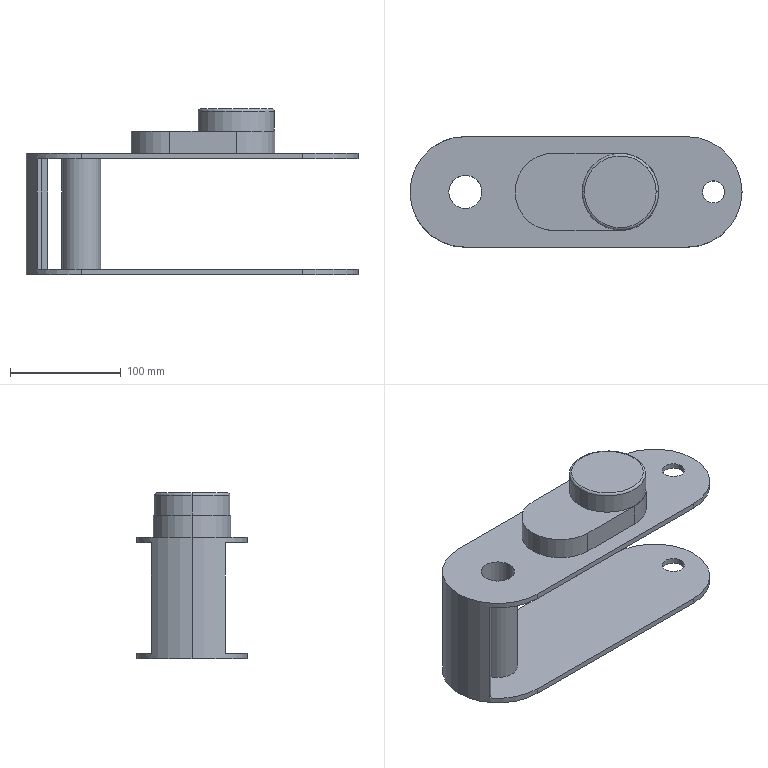Part | SolidWorks | features ICE 7, Extrusion 1, Fillet 1 | 1 solid | 41 faces | box 300 x 100 x 150 mm | volume 561268 mm3 | cylinder 23 | plane 16 | torus 2 | commonest cylinder face diameters 20 x8 100 x4 70 x3 30 x2 35 x2 69 x2
STEP:
#1=CARTESIAN_POINT('',(105.5,0.,148.));
#2=VERTEX_POINT('',#1);
#3=CARTESIAN_POINT('',(174.5,0.,148.));
#4=VERTEX_POINT('',#3);
#5=CARTESIAN_POINT('',(140.,0.,148.));
#6=DIRECTION('',(0.,0.,-1.));
#7=DIRECTION('',(1.,0.,0.));
#8=AXIS2_PLACEMENT_3D('',#5,#6,#7);
#9=CIRCLE('',#8,34.5);
#10=EDGE_CURVE('',#2,#4,#9,.T.);
#11=ORIENTED_EDGE('',*,*,#10,.F.);
#12=CARTESIAN_POINT('',(107.5,0.,150.));
#13=VERTEX_POINT('',#12);
#14=CARTESIAN_POINT('',(107.5,0.,148.));
#15=DIRECTION('',(0.,1.,0.));
#16=DIRECTION('',(-1.,0.,0.));
#17=AXIS2_PLACEMENT_3D('',#14,#15,#16);
#18=CIRCLE('',#17,2.);
#19=EDGE_CURVE('',#2,#13,#18,.T.);
#20=ORIENTED_EDGE('',*,*,#19,.T.);
#21=CARTESIAN_POINT('',(172.5,0.,150.));
#22=VERTEX_POINT('',#21);
#23=CARTESIAN_POINT('',(140.,0.,150.));
#24=DIRECTION('',(0.,0.,1.));
#25=DIRECTION('',(1.,0.,0.));
#26=AXIS2_PLACEMENT_3D('',#23,#24,#25);
#27=CIRCLE('',#26,32.5);
#28=EDGE_CURVE('',#22,#13,#27,.T.);
#29=ORIENTED_EDGE('',*,*,#28,.F.);
#30=CARTESIAN_POINT('',(172.5,0.,148.));
#31=DIRECTION('',(0.,-1.,0.));
#32=DIRECTION('',(0.,0.,-1.));
#33=AXIS2_PLACEMENT_3D('',#30,#31,#32);
#34=CIRCLE('',#33,2.);
#35=EDGE_CURVE('',#4,#22,#34,.T.);
#36=ORIENTED_EDGE('',*,*,#35,.F.);
#37=EDGE_LOOP('',(#11,#20,#29,#36));
#38=FACE_OUTER_BOUND('',#37,.T.);
#39=CARTESIAN_POINT('',(140.,0.,148.));
#40=DIRECTION('',(0.,0.,1.));
#41=DIRECTION('',(1.,0.,0.));
#42=AXIS2_PLACEMENT_3D('',#39,#40,#41);
#43=TOROIDAL_SURFACE('',#42,32.5,2.);
#44=ADVANCED_FACE('',(#38),#43,.T.);
#45=CARTESIAN_POINT('',(-45.,0.,105.));
#46=VERTEX_POINT('',#45);
#47=CARTESIAN_POINT('',(-30.342,33.232,105.));
#48=VERTEX_POINT('',#47);
#49=CARTESIAN_POINT('',(0.,0.,105.));
#50=DIRECTION('',(0.,0.,-1.));
#51=DIRECTION('',(1.,0.,0.));
#52=AXIS2_PLACEMENT_3D('',#49,#50,#51);
#53=CIRCLE('',#52,45.);
#54=EDGE_CURVE('',#46,#48,#53,.T.);
#55=ORIENTED_EDGE('',*,*,#54,.F.);
#56=CARTESIAN_POINT('',(-45.,0.,5.));
#57=VERTEX_POINT('',#56);
#58=CARTESIAN_POINT('',(-45.,0.,150.002));
#59=DIRECTION('',(0.,0.,-1.));
#60=VECTOR('',#59,1000.);
#61=LINE('',#58,#60);
#62=EDGE_CURVE('',#46,#57,#61,.T.);
#63=ORIENTED_EDGE('',*,*,#62,.T.);
#64=CARTESIAN_POINT('',(-30.342,33.232,5.));
#65=VERTEX_POINT('',#64);
#66=CARTESIAN_POINT('',(0.,0.,5.));
#67=DIRECTION('',(0.,0.,-1.));
#68=DIRECTION('',(1.,0.,0.));
#69=AXIS2_PLACEMENT_3D('',#66,#67,#68);
#70=CIRCLE('',#69,45.);
#71=EDGE_CURVE('',#57,#65,#70,.T.);
#72=ORIENTED_EDGE('',*,*,#71,.T.);
#73=CARTESIAN_POINT('',(-30.342,33.232,150.002));
#74=DIRECTION('',(0.,0.,-1.));
#75=VECTOR('',#74,1000.);
#76=LINE('',#73,#75);
#77=EDGE_CURVE('',#48,#65,#76,.T.);
#78=ORIENTED_EDGE('',*,*,#77,.F.);
#79=EDGE_LOOP('',(#55,#63,#72,#78));
#80=FACE_OUTER_BOUND('',#79,.T.);
#81=CARTESIAN_POINT('',(0.,0.,150.002));
#82=DIRECTION('',(0.,0.,-1.));
#83=DIRECTION('',(-1.,0.,0.));
#84=AXIS2_PLACEMENT_3D('',#81,#82,#83);
#85=CYLINDRICAL_SURFACE('',#84,45.);
#86=ADVANCED_FACE('',(#80),#85,.F.);
#87=CARTESIAN_POINT('',(214.307,0.,5.));
#88=VERTEX_POINT('',#87);
#89=CARTESIAN_POINT('',(234.307,0.,5.));
#90=VERTEX_POINT('',#89);
#91=CARTESIAN_POINT('',(224.307,0.,5.));
#92=DIRECTION('',(0.,0.,1.));
#93=DIRECTION('',(1.,0.,0.));
#94=AXIS2_PLACEMENT_3D('',#91,#92,#93);
#95=CIRCLE('',#94,10.);
#96=EDGE_CURVE('',#88,#90,#95,.T.);
#97=ORIENTED_EDGE('',*,*,#96,.T.);
#98=CARTESIAN_POINT('',(234.307,0.,0.));
#99=VERTEX_POINT('',#98);
#100=CARTESIAN_POINT('',(234.307,0.,127.));
#101=DIRECTION('',(0.,0.,-1.));
#102=VECTOR('',#101,1000.);
#103=LINE('',#100,#102);
#104=EDGE_CURVE('',#90,#99,#103,.T.);
#105=ORIENTED_EDGE('',*,*,#104,.T.);
#106=CARTESIAN_POINT('',(214.307,0.,0.));
#107=VERTEX_POINT('',#106);
#108=CARTESIAN_POINT('',(224.307,0.,0.));
#109=DIRECTION('',(0.,0.,-1.));
#110=DIRECTION('',(-1.,0.,0.));
#111=AXIS2_PLACEMENT_3D('',#108,#109,#110);
#112=CIRCLE('',#111,10.);
#113=EDGE_CURVE('',#99,#107,#112,.T.);
#114=ORIENTED_EDGE('',*,*,#113,.T.);
#115=CARTESIAN_POINT('',(214.307,0.,127.));
#116=DIRECTION('',(0.,0.,-1.));
#117=VECTOR('',#116,1000.);
#118=LINE('',#115,#117);
#119=EDGE_CURVE('',#88,#107,#118,.T.);
#120=ORIENTED_EDGE('',*,*,#119,.F.);
#121=EDGE_LOOP('',(#97,#105,#114,#120));
#122=FACE_OUTER_BOUND('',#121,.T.);
#123=CARTESIAN_POINT('',(224.307,0.,127.));
#124=DIRECTION('',(0.,0.,-1.));
#125=DIRECTION('',(-1.,0.,0.));
#126=AXIS2_PLACEMENT_3D('',#123,#124,#125);
#127=CYLINDRICAL_SURFACE('',#126,10.);
#128=ADVANCED_FACE('',(#122),#127,.F.);
#129=CARTESIAN_POINT('',(214.307,0.,110.));
#130=VERTEX_POINT('',#129);
#131=CARTESIAN_POINT('',(234.307,0.,110.));
#132=VERTEX_POINT('',#131);
#133=CARTESIAN_POINT('',(224.307,0.,110.));
#134=DIRECTION('',(0.,0.,1.));
#135=DIRECTION('',(1.,0.,0.));
#136=AXIS2_PLACEMENT_3D('',#133,#134,#135);
#137=CIRCLE('',#136,10.);
#138=EDGE_CURVE('',#130,#132,#137,.T.);
#139=ORIENTED_EDGE('',*,*,#138,.T.);
#140=CARTESIAN_POINT('',(234.307,0.,105.));
#141=VERTEX_POINT('',#140);
#142=CARTESIAN_POINT('',(234.307,0.,127.));
#143=DIRECTION('',(0.,0.,-1.));
#144=VECTOR('',#143,1000.);
#145=LINE('',#142,#144);
#146=EDGE_CURVE('',#132,#141,#145,.T.);
#147=ORIENTED_EDGE('',*,*,#146,.T.);
#148=CARTESIAN_POINT('',(214.307,0.,105.));
#149=VERTEX_POINT('',#148);
#150=CARTESIAN_POINT('',(224.307,0.,105.));
#151=DIRECTION('',(0.,0.,1.));
#152=DIRECTION('',(1.,0.,0.));
#153=AXIS2_PLACEMENT_3D('',#150,#151,#152);
#154=CIRCLE('',#153,10.);
#155=EDGE_CURVE('',#149,#141,#154,.T.);
#156=ORIENTED_EDGE('',*,*,#155,.F.);
#157=CARTESIAN_POINT('',(214.307,0.,127.));
#158=DIRECTION('',(0.,0.,-1.));
#159=VECTOR('',#158,1000.);
#160=LINE('',#157,#159);
#161=EDGE_CURVE('',#130,#149,#160,.T.);
#162=ORIENTED_EDGE('',*,*,#161,.F.);
#163=EDGE_LOOP('',(#139,#147,#156,#162));
#164=FACE_OUTER_BOUND('',#163,.T.);
#165=CARTESIAN_POINT('',(224.307,0.,127.));
#166=DIRECTION('',(0.,0.,-1.));
#167=DIRECTION('',(-1.,0.,0.));
#168=AXIS2_PLACEMENT_3D('',#165,#166,#167);
#169=CYLINDRICAL_SURFACE('',#168,10.);
#170=ADVANCED_FACE('',(#164),#169,.F.);
#171=ORIENTED_EDGE('',*,*,#10,.T.);
#172=CARTESIAN_POINT('',(174.5,0.,130.));
#173=VERTEX_POINT('',#172);
#174=CARTESIAN_POINT('',(174.5,0.,150.));
#175=DIRECTION('',(0.,0.,-1.));
#176=VECTOR('',#175,1000.);
#177=LINE('',#174,#176);
#178=EDGE_CURVE('',#4,#173,#177,.T.);
#179=ORIENTED_EDGE('',*,*,#178,.T.);
#180=CARTESIAN_POINT('',(105.5,0.,130.));
#181=VERTEX_POINT('',#180);
#182=CARTESIAN_POINT('',(140.,0.,130.));
#183=DIRECTION('',(0.,0.,1.));
#184=DIRECTION('',(1.,0.,0.));
#185=AXIS2_PLACEMENT_3D('',#182,#183,#184);
#186=CIRCLE('',#185,34.5);
#187=EDGE_CURVE('',#173,#181,#186,.T.);
#188=ORIENTED_EDGE('',*,*,#187,.T.);
#189=CARTESIAN_POINT('',(105.5,0.,150.));
#190=DIRECTION('',(0.,0.,-1.));
#191=VECTOR('',#190,1000.);
#192=LINE('',#189,#191);
#193=EDGE_CURVE('',#2,#181,#192,.T.);
#194=ORIENTED_EDGE('',*,*,#193,.F.);
#195=EDGE_LOOP('',(#171,#179,#188,#194));
#196=FACE_OUTER_BOUND('',#195,.T.);
#197=CARTESIAN_POINT('',(140.,0.,150.));
#198=DIRECTION('',(0.,0.,-1.));
#199=DIRECTION('',(-1.,0.,0.));
#200=AXIS2_PLACEMENT_3D('',#197,#198,#199);
#201=CYLINDRICAL_SURFACE('',#200,34.5);
#202=ADVANCED_FACE('',(#196),#201,.T.);
#203=CARTESIAN_POINT('',(45.,0.,130.));
#204=VERTEX_POINT('',#203);
#205=CARTESIAN_POINT('',(80.,-35.,130.));
#206=VERTEX_POINT('',#205);
#207=CARTESIAN_POINT('',(80.,0.,130.));
#208=DIRECTION('',(0.,0.,1.));
#209=DIRECTION('',(1.,0.,0.));
#210=AXIS2_PLACEMENT_3D('',#207,#208,#209);
#211=CIRCLE('',#210,35.);
#212=EDGE_CURVE('',#204,#206,#211,.T.);
#213=ORIENTED_EDGE('',*,*,#212,.F.);
#214=CARTESIAN_POINT('',(45.,0.,110.));
#215=VERTEX_POINT('',#214);
#216=CARTESIAN_POINT('',(45.,0.,130.));
#217=DIRECTION('',(0.,0.,-1.));
#218=VECTOR('',#217,1000.);
#219=LINE('',#216,#218);
#220=EDGE_CURVE('',#204,#215,#219,.T.);
#221=ORIENTED_EDGE('',*,*,#220,.T.);
#222=CARTESIAN_POINT('',(80.,-35.,110.));
#223=VERTEX_POINT('',#222);
#224=CARTESIAN_POINT('',(80.,0.,110.));
#225=DIRECTION('',(0.,0.,1.));
#226=DIRECTION('',(1.,0.,0.));
#227=AXIS2_PLACEMENT_3D('',#224,#225,#226);
#228=CIRCLE('',#227,35.);
#229=EDGE_CURVE('',#215,#223,#228,.T.);
#230=ORIENTED_EDGE('',*,*,#229,.T.);
#231=CARTESIAN_POINT('',(80.,-35.,130.));
#232=DIRECTION('',(0.,0.,-1.));
#233=VECTOR('',#232,1000.);
#234=LINE('',#231,#233);
#235=EDGE_CURVE('',#206,#223,#234,.T.);
#236=ORIENTED_EDGE('',*,*,#235,.F.);
#237=EDGE_LOOP('',(#213,#221,#230,#236));
#238=FACE_OUTER_BOUND('',#237,.T.);
#239=CARTESIAN_POINT('',(80.,0.,130.));
#240=DIRECTION('',(0.,0.,-1.));
#241=DIRECTION('',(-1.,0.,0.));
#242=AXIS2_PLACEMENT_3D('',#239,#240,#241);
#243=CYLINDRICAL_SURFACE('',#242,35.);
#244=ADVANCED_FACE('',(#238),#243,.T.);
#245=CARTESIAN_POINT('',(130.,0.,110.));
#246=VERTEX_POINT('',#245);
#247=CARTESIAN_POINT('',(150.,0.,110.));
#248=VERTEX_POINT('',#247);
#249=CARTESIAN_POINT('',(140.,0.,110.));
#250=DIRECTION('',(0.,0.,1.));
#251=DIRECTION('',(1.,0.,0.));
#252=AXIS2_PLACEMENT_3D('',#249,#250,#251);
#253=CIRCLE('',#252,10.);
#254=EDGE_CURVE('',#246,#248,#253,.T.);
#255=ORIENTED_EDGE('',*,*,#254,.T.);
#256=CARTESIAN_POINT('',(150.,0.,105.));
#257=VERTEX_POINT('',#256);
#258=CARTESIAN_POINT('',(150.,0.,151.));
#259=DIRECTION('',(0.,0.,-1.));
#260=VECTOR('',#259,1000.);
#261=LINE('',#258,#260);
#262=EDGE_CURVE('',#248,#257,#261,.T.);
#263=ORIENTED_EDGE('',*,*,#262,.T.);
#264=CARTESIAN_POINT('',(130.,0.,105.));
#265=VERTEX_POINT('',#264);
#266=CARTESIAN_POINT('',(140.,0.,105.));
#267=DIRECTION('',(0.,0.,-1.));
#268=DIRECTION('',(-1.,0.,0.));
#269=AXIS2_PLACEMENT_3D('',#266,#267,#268);
#270=CIRCLE('',#269,10.);
#271=EDGE_CURVE('',#257,#265,#270,.T.);
#272=ORIENTED_EDGE('',*,*,#271,.T.);
#273=CARTESIAN_POINT('',(130.,0.,151.));
#274=DIRECTION('',(0.,0.,-1.));
#275=VECTOR('',#274,1000.);
#276=LINE('',#273,#275);
#277=EDGE_CURVE('',#246,#265,#276,.T.);
#278=ORIENTED_EDGE('',*,*,#277,.F.);
#279=EDGE_LOOP('',(#255,#263,#272,#278));
#280=FACE_OUTER_BOUND('',#279,.T.);
#281=CARTESIAN_POINT('',(140.,0.,151.));
#282=DIRECTION('',(0.,0.,-1.));
#283=DIRECTION('',(-1.,0.,0.));
#284=AXIS2_PLACEMENT_3D('',#281,#282,#283);
#285=CYLINDRICAL_SURFACE('',#284,10.);
#286=ADVANCED_FACE('',(#280),#285,.F.);
#287=CARTESIAN_POINT('',(70.,0.,110.));
#288=VERTEX_POINT('',#287);
#289=CARTESIAN_POINT('',(90.,0.,110.));
#290=VERTEX_POINT('',#289);
#291=CARTESIAN_POINT('',(80.,0.,110.));
#292=DIRECTION('',(0.,0.,1.));
#293=DIRECTION('',(1.,0.,0.));
#294=AXIS2_PLACEMENT_3D('',#291,#292,#293);
#295=CIRCLE('',#294,10.);
#296=EDGE_CURVE('',#288,#290,#295,.T.);
#297=ORIENTED_EDGE('',*,*,#296,.T.);
#298=CARTESIAN_POINT('',(90.,0.,105.));
#299=VERTEX_POINT('',#298);
#300=CARTESIAN_POINT('',(90.,0.,151.));
#301=DIRECTION('',(0.,0.,-1.));
#302=VECTOR('',#301,1000.);
#303=LINE('',#300,#302);
#304=EDGE_CURVE('',#290,#299,#303,.T.);
#305=ORIENTED_EDGE('',*,*,#304,.T.);
#306=CARTESIAN_POINT('',(70.,0.,105.));
#307=VERTEX_POINT('',#306);
#308=CARTESIAN_POINT('',(80.,0.,105.));
#309=DIRECTION('',(0.,0.,-1.));
#310=DIRECTION('',(-1.,0.,0.));
#311=AXIS2_PLACEMENT_3D('',#308,#309,#310);
#312=CIRCLE('',#311,10.);
#313=EDGE_CURVE('',#299,#307,#312,.T.);
#314=ORIENTED_EDGE('',*,*,#313,.T.);
#315=CARTESIAN_POINT('',(70.,0.,151.));
#316=DIRECTION('',(0.,0.,-1.));
#317=VECTOR('',#316,1000.);
#318=LINE('',#315,#317);
#319=EDGE_CURVE('',#288,#307,#318,.T.);
#320=ORIENTED_EDGE('',*,*,#319,.F.);
#321=EDGE_LOOP('',(#297,#305,#314,#320));
#322=FACE_OUTER_BOUND('',#321,.T.);
#323=CARTESIAN_POINT('',(80.,0.,151.));
#324=DIRECTION('',(0.,0.,-1.));
#325=DIRECTION('',(-1.,0.,0.));
#326=AXIS2_PLACEMENT_3D('',#323,#324,#325);
#327=CYLINDRICAL_SURFACE('',#326,10.);
#328=ADVANCED_FACE('',(#322),#327,.F.);
#329=CARTESIAN_POINT('',(17.5,0.,105.));
#330=VERTEX_POINT('',#329);
#331=CARTESIAN_POINT('',(-17.5,0.,105.));
#332=VERTEX_POINT('',#331);
#333=CARTESIAN_POINT('',(0.,0.,105.));
#334=DIRECTION('',(0.,0.,1.));
#335=DIRECTION('',(1.,0.,0.));
#336=AXIS2_PLACEMENT_3D('',#333,#334,#335);
#337=CIRCLE('',#336,17.5);
#338=EDGE_CURVE('',#330,#332,#337,.T.);
#339=ORIENTED_EDGE('',*,*,#338,.F.);
#340=CARTESIAN_POINT('',(17.5,0.,5.));
#341=VERTEX_POINT('',#340);
#342=CARTESIAN_POINT('',(17.5,0.,154.497));
#343=DIRECTION('',(0.,0.,-1.));
#344=VECTOR('',#343,1000.);
#345=LINE('',#342,#344);
#346=EDGE_CURVE('',#330,#341,#345,.T.);
#347=ORIENTED_EDGE('',*,*,#346,.T.);
#348=CARTESIAN_POINT('',(-17.5,0.,5.));
#349=VERTEX_POINT('',#348);
#350=CARTESIAN_POINT('',(0.,0.,5.));
#351=DIRECTION('',(0.,0.,1.));
#352=DIRECTION('',(1.,0.,0.));
#353=AXIS2_PLACEMENT_3D('',#350,#351,#352);
#354=CIRCLE('',#353,17.5);
#355=EDGE_CURVE('',#341,#349,#354,.T.);
#356=ORIENTED_EDGE('',*,*,#355,.T.);
#357=CARTESIAN_POINT('',(-17.5,0.,154.497));
#358=DIRECTION('',(0.,0.,-1.));
#359=VECTOR('',#358,1000.);
#360=LINE('',#357,#359);
#361=EDGE_CURVE('',#332,#349,#360,.T.);
#362=ORIENTED_EDGE('',*,*,#361,.F.);
#363=EDGE_LOOP('',(#339,#347,#356,#362));
#364=FACE_OUTER_BOUND('',#363,.T.);
#365=CARTESIAN_POINT('',(0.,0.,154.497));
#366=DIRECTION('',(0.,0.,-1.));
#367=DIRECTION('',(-1.,0.,0.));
#368=AXIS2_PLACEMENT_3D('',#365,#366,#367);
#369=CYLINDRICAL_SURFACE('',#368,17.5);
#370=ADVANCED_FACE('',(#364),#369,.T.);
#371=CARTESIAN_POINT('',(-15.,0.,110.));
#372=VERTEX_POINT('',#371);
#373=CARTESIAN_POINT('',(15.,0.,110.));
#374=VERTEX_POINT('',#373);
#375=CARTESIAN_POINT('',(0.,0.,110.));
#376=DIRECTION('',(0.,0.,1.));
#377=DIRECTION('',(1.,0.,0.));
#378=AXIS2_PLACEMENT_3D('',#375,#376,#377);
#379=CIRCLE('',#378,15.);
#380=EDGE_CURVE('',#372,#374,#379,.T.);
#381=ORIENTED_EDGE('',*,*,#380,.T.);
#382=CARTESIAN_POINT('',(15.,0.,0.));
#383=VERTEX_POINT('',#382);
#384=CARTESIAN_POINT('',(15.,0.,5.));
#385=DIRECTION('',(0.,0.,-1.));
#386=VECTOR('',#385,1000.);
#387=LINE('',#384,#386);
#388=EDGE_CURVE('',#374,#383,#387,.T.);
#389=ORIENTED_EDGE('',*,*,#388,.T.);
#390=CARTESIAN_POINT('',(-15.,0.,0.));
#391=VERTEX_POINT('',#390);
#392=CARTESIAN_POINT('',(0.,0.,0.));
#393=DIRECTION('',(0.,0.,1.));
#394=DIRECTION('',(1.,0.,0.));
#395=AXIS2_PLACEMENT_3D('',#392,#393,#394);
#396=CIRCLE('',#395,15.);
#397=EDGE_CURVE('',#391,#383,#396,.T.);
#398=ORIENTED_EDGE('',*,*,#397,.F.);
#399=CARTESIAN_POINT('',(-15.,0.,5.));
#400=DIRECTION('',(0.,0.,-1.));
#401=VECTOR('',#400,1000.);
#402=LINE('',#399,#401);
#403=EDGE_CURVE('',#372,#391,#402,.T.);
#404=ORIENTED_EDGE('',*,*,#403,.F.);
#405=EDGE_LOOP('',(#381,#389,#398,#404));
#406=FACE_OUTER_BOUND('',#405,.T.);
#407=CARTESIAN_POINT('',(0.,0.,5.));
#408=DIRECTION('',(0.,0.,-1.));
#409=DIRECTION('',(-1.,0.,0.));
#410=AXIS2_PLACEMENT_3D('',#407,#408,#409);
#411=CYLINDRICAL_SURFACE('',#410,15.);
#412=ADVANCED_FACE('',(#406),#411,.F.);
#413=CARTESIAN_POINT('',(-50.,0.,110.));
#414=VERTEX_POINT('',#413);
#415=CARTESIAN_POINT('',(0.,-50.,110.));
#416=VERTEX_POINT('',#415);
#417=CARTESIAN_POINT('',(0.,0.,110.));
#418=DIRECTION('',(0.,0.,1.));
#419=DIRECTION('',(1.,0.,0.));
#420=AXIS2_PLACEMENT_3D('',#417,#418,#419);
#421=CIRCLE('',#420,50.);
#422=EDGE_CURVE('',#414,#416,#421,.T.);
#423=ORIENTED_EDGE('',*,*,#422,.F.);
#424=CARTESIAN_POINT('',(-50.,0.,0.));
#425=VERTEX_POINT('',#424);
#426=CARTESIAN_POINT('',(-50.,0.,5.));
#427=DIRECTION('',(0.,0.,-1.));
#428=VECTOR('',#427,1000.);
#429=LINE('',#426,#428);
#430=EDGE_CURVE('',#414,#425,#429,.T.);
#431=ORIENTED_EDGE('',*,*,#430,.T.);
#432=CARTESIAN_POINT('',(0.,-50.,0.));
#433=VERTEX_POINT('',#432);
#434=CARTESIAN_POINT('',(0.,0.,0.));
#435=DIRECTION('',(0.,0.,1.));
#436=DIRECTION('',(1.,0.,0.));
#437=AXIS2_PLACEMENT_3D('',#434,#435,#436);
#438=CIRCLE('',#437,50.);
#439=EDGE_CURVE('',#425,#433,#438,.T.);
#440=ORIENTED_EDGE('',*,*,#439,.T.);
#441=CARTESIAN_POINT('',(0.,-50.,5.));
#442=VERTEX_POINT('',#441);
#443=CARTESIAN_POINT('',(0.,-50.,5.));
#444=DIRECTION('',(0.,0.,-1.));
#445=VECTOR('',#444,1000.);
#446=LINE('',#443,#445);
#447=EDGE_CURVE('',#442,#433,#446,.T.);
#448=ORIENTED_EDGE('',*,*,#447,.F.);
#449=CARTESIAN_POINT('',(-40.04,-29.947,5.));
#450=VERTEX_POINT('',#449);
#451=CARTESIAN_POINT('',(0.,0.,5.));
#452=DIRECTION('',(0.,0.,1.));
#453=DIRECTION('',(1.,0.,0.));
#454=AXIS2_PLACEMENT_3D('',#451,#452,#453);
#455=CIRCLE('',#454,50.);
#456=EDGE_CURVE('',#450,#442,#455,.T.);
#457=ORIENTED_EDGE('',*,*,#456,.F.);
#458=CARTESIAN_POINT('',(-40.04,-29.947,105.));
#459=VERTEX_POINT('',#458);
#460=CARTESIAN_POINT('',(-40.04,-29.947,150.002));
#461=DIRECTION('',(0.,0.,-1.));
#462=VECTOR('',#461,1000.);
#463=LINE('',#460,#462);
#464=EDGE_CURVE('',#459,#450,#463,.T.);
#465=ORIENTED_EDGE('',*,*,#464,.F.);
#466=CARTESIAN_POINT('',(0.,-50.,105.));
#467=VERTEX_POINT('',#466);
#468=CARTESIAN_POINT('',(0.,0.,105.));
#469=DIRECTION('',(0.,0.,1.));
#470=DIRECTION('',(1.,0.,0.));
#471=AXIS2_PLACEMENT_3D('',#468,#469,#470);
#472=CIRCLE('',#471,50.);
#473=EDGE_CURVE('',#459,#467,#472,.T.);
#474=ORIENTED_EDGE('',*,*,#473,.T.);
#475=CARTESIAN_POINT('',(0.,-50.,110.));
#476=DIRECTION('',(0.,0.,-1.));
#477=VECTOR('',#476,1000.);
#478=LINE('',#475,#477);
#479=EDGE_CURVE('',#416,#467,#478,.T.);
#480=ORIENTED_EDGE('',*,*,#479,.F.);
#481=EDGE_LOOP('',(#423,#431,#440,#448,#457,#465,#474,#480));
#482=FACE_OUTER_BOUND('',#481,.T.);
#483=CARTESIAN_POINT('',(0.,0.,5.));
#484=DIRECTION('',(0.,0.,-1.));
#485=DIRECTION('',(-1.,0.,0.));
#486=AXIS2_PLACEMENT_3D('',#483,#484,#485);
#487=CYLINDRICAL_SURFACE('',#486,50.);
#488=ADVANCED_FACE('',(#482),#487,.T.);
#489=ORIENTED_EDGE('',*,*,#96,.F.);
#490=CARTESIAN_POINT('',(224.307,0.,5.));
#491=DIRECTION('',(0.,0.,1.));
#492=DIRECTION('',(1.,0.,0.));
#493=AXIS2_PLACEMENT_3D('',#490,#491,#492);
#494=CIRCLE('',#493,10.);
#495=EDGE_CURVE('',#90,#88,#494,.T.);
#496=ORIENTED_EDGE('',*,*,#495,.F.);
#497=EDGE_LOOP('',(#489,#496));
#498=FACE_BOUND('',#497,.T.);
#499=CARTESIAN_POINT('',(0.,0.,5.));
#500=DIRECTION('',(0.,0.,1.));
#501=DIRECTION('',(1.,0.,0.));
#502=AXIS2_PLACEMENT_3D('',#499,#500,#501);
#503=CIRCLE('',#502,17.5);
#504=EDGE_CURVE('',#349,#341,#503,.T.);
#505=ORIENTED_EDGE('',*,*,#504,.F.);
#506=ORIENTED_EDGE('',*,*,#355,.F.);
#507=EDGE_LOOP('',(#505,#506));
#508=FACE_BOUND('',#507,.T.);
#509=CARTESIAN_POINT('',(-36.036,-26.952,5.));
#510=VERTEX_POINT('',#509);
#511=CARTESIAN_POINT('',(0.,0.,5.));
#512=DIRECTION('',(0.,0.,-1.));
#513=DIRECTION('',(1.,0.,0.));
#514=AXIS2_PLACEMENT_3D('',#511,#512,#513);
#515=CIRCLE('',#514,45.);
#516=EDGE_CURVE('',#510,#57,#515,.T.);
#517=ORIENTED_EDGE('',*,*,#516,.F.);
#518=CARTESIAN_POINT('',(-40.04,-29.947,5.));
#519=DIRECTION('',(0.8008,0.5989,0.));
#520=VECTOR('',#519,1000.);
#521=LINE('',#518,#520);
#522=EDGE_CURVE('',#450,#510,#521,.T.);
#523=ORIENTED_EDGE('',*,*,#522,.F.);
#524=ORIENTED_EDGE('',*,*,#456,.T.);
#525=CARTESIAN_POINT('',(200.,-50.,5.));
#526=VERTEX_POINT('',#525);
#527=CARTESIAN_POINT('',(0.,-50.,5.));
#528=DIRECTION('',(1.,0.,0.));
#529=VECTOR('',#528,1000.);
#530=LINE('',#527,#529);
#531=EDGE_CURVE('',#442,#526,#530,.T.);
#532=ORIENTED_EDGE('',*,*,#531,.T.);
#533=CARTESIAN_POINT('',(200.,50.,5.));
#534=VERTEX_POINT('',#533);
#535=CARTESIAN_POINT('',(200.,0.,5.));
#536=DIRECTION('',(0.,0.,1.));
#537=DIRECTION('',(1.,0.,0.));
#538=AXIS2_PLACEMENT_3D('',#535,#536,#537);
#539=CIRCLE('',#538,50.);
#540=EDGE_CURVE('',#526,#534,#539,.T.);
#541=ORIENTED_EDGE('',*,*,#540,.T.);
#542=CARTESIAN_POINT('',(0.,50.,5.));
#543=VERTEX_POINT('',#542);
#544=CARTESIAN_POINT('',(0.,50.,5.));
#545=DIRECTION('',(-1.,0.,0.));
#546=VECTOR('',#545,1000.);
#547=LINE('',#544,#546);
#548=EDGE_CURVE('',#534,#543,#547,.T.);
#549=ORIENTED_EDGE('',*,*,#548,.T.);
#550=CARTESIAN_POINT('',(-33.713,36.925,5.));
#551=VERTEX_POINT('',#550);
#552=CARTESIAN_POINT('',(0.,0.,5.));
#553=DIRECTION('',(0.,0.,1.));
#554=DIRECTION('',(1.,0.,0.));
#555=AXIS2_PLACEMENT_3D('',#552,#553,#554);
#556=CIRCLE('',#555,50.);
#557=EDGE_CURVE('',#543,#551,#556,.T.);
#558=ORIENTED_EDGE('',*,*,#557,.T.);
#559=CARTESIAN_POINT('',(-33.713,36.925,5.));
#560=DIRECTION('',(-0.6743,0.7385,0.));
#561=VECTOR('',#560,1000.);
#562=LINE('',#559,#561);
#563=EDGE_CURVE('',#65,#551,#562,.T.);
#564=ORIENTED_EDGE('',*,*,#563,.F.);
#565=ORIENTED_EDGE('',*,*,#71,.F.);
#566=EDGE_LOOP('',(#517,#523,#524,#532,#541,#549,#558,#564,#565));
#567=FACE_OUTER_BOUND('',#566,.T.);
#568=CARTESIAN_POINT('',(0.,0.,5.));
#569=DIRECTION('',(0.,0.,1.));
#570=DIRECTION('',(1.,0.,0.));
#571=AXIS2_PLACEMENT_3D('',#568,#569,#570);
#572=PLANE('',#571);
#573=ADVANCED_FACE('',(#498,#508,#567),#572,.T.);
#574=CARTESIAN_POINT('',(0.,0.,105.));
#575=DIRECTION('',(0.,0.,1.));
#576=DIRECTION('',(1.,0.,0.));
#577=AXIS2_PLACEMENT_3D('',#574,#575,#576);
#578=CIRCLE('',#577,17.5);
#579=EDGE_CURVE('',#332,#330,#578,.T.);
#580=ORIENTED_EDGE('',*,*,#579,.T.);
#581=ORIENTED_EDGE('',*,*,#338,.T.);
#582=EDGE_LOOP('',(#580,#581));
#583=FACE_BOUND('',#582,.T.);
#584=CARTESIAN_POINT('',(80.,0.,105.));
#585=DIRECTION('',(0.,0.,-1.));
#586=DIRECTION('',(-1.,0.,0.));
#587=AXIS2_PLACEMENT_3D('',#584,#585,#586);
#588=CIRCLE('',#587,10.);
#589=EDGE_CURVE('',#307,#299,#588,.T.);
#590=ORIENTED_EDGE('',*,*,#589,.F.);
#591=ORIENTED_EDGE('',*,*,#313,.F.);
#592=EDGE_LOOP('',(#590,#591));
#593=FACE_BOUND('',#592,.T.);
#594=CARTESIAN_POINT('',(140.,0.,105.));
#595=DIRECTION('',(0.,0.,-1.));
#596=DIRECTION('',(-1.,0.,0.));
#597=AXIS2_PLACEMENT_3D('',#594,#595,#596);
#598=CIRCLE('',#597,10.);
#599=EDGE_CURVE('',#265,#257,#598,.T.);
#600=ORIENTED_EDGE('',*,*,#599,.F.);
#601=ORIENTED_EDGE('',*,*,#271,.F.);
#602=EDGE_LOOP('',(#600,#601));
#603=FACE_BOUND('',#602,.T.);
#604=ORIENTED_EDGE('',*,*,#155,.T.);
#605=CARTESIAN_POINT('',(224.307,0.,105.));
#606=DIRECTION('',(0.,0.,1.));
#607=DIRECTION('',(1.,0.,0.));
#608=AXIS2_PLACEMENT_3D('',#605,#606,#607);
#609=CIRCLE('',#608,10.);
#610=EDGE_CURVE('',#141,#149,#609,.T.);
#611=ORIENTED_EDGE('',*,*,#610,.T.);
#612=EDGE_LOOP('',(#604,#611));
#613=FACE_BOUND('',#612,.T.);
#614=CARTESIAN_POINT('',(-36.036,-26.952,105.));
#615=VERTEX_POINT('',#614);
#616=CARTESIAN_POINT('',(-40.04,-29.947,105.));
#617=DIRECTION('',(0.8008,0.5989,0.));
#618=VECTOR('',#617,1000.);
#619=LINE('',#616,#618);
#620=EDGE_CURVE('',#459,#615,#619,.T.);
#621=ORIENTED_EDGE('',*,*,#620,.T.);
#622=CARTESIAN_POINT('',(0.,0.,105.));
#623=DIRECTION('',(0.,0.,-1.));
#624=DIRECTION('',(1.,0.,0.));
#625=AXIS2_PLACEMENT_3D('',#622,#623,#624);
#626=CIRCLE('',#625,45.);
#627=EDGE_CURVE('',#615,#46,#626,.T.);
#628=ORIENTED_EDGE('',*,*,#627,.T.);
#629=ORIENTED_EDGE('',*,*,#54,.T.);
#630=CARTESIAN_POINT('',(-33.713,36.925,105.));
#631=VERTEX_POINT('',#630);
#632=CARTESIAN_POINT('',(-33.713,36.925,105.));
#633=DIRECTION('',(-0.6743,0.7385,0.));
#634=VECTOR('',#633,1000.);
#635=LINE('',#632,#634);
#636=EDGE_CURVE('',#48,#631,#635,.T.);
#637=ORIENTED_EDGE('',*,*,#636,.T.);
#638=CARTESIAN_POINT('',(0.,50.,105.));
#639=VERTEX_POINT('',#638);
#640=CARTESIAN_POINT('',(0.,0.,105.));
#641=DIRECTION('',(0.,0.,1.));
#642=DIRECTION('',(1.,0.,0.));
#643=AXIS2_PLACEMENT_3D('',#640,#641,#642);
#644=CIRCLE('',#643,50.);
#645=EDGE_CURVE('',#639,#631,#644,.T.);
#646=ORIENTED_EDGE('',*,*,#645,.F.);
#647=CARTESIAN_POINT('',(200.,50.,105.));
#648=VERTEX_POINT('',#647);
#649=CARTESIAN_POINT('',(200.,50.,105.));
#650=DIRECTION('',(-1.,0.,0.));
#651=VECTOR('',#650,1000.);
#652=LINE('',#649,#651);
#653=EDGE_CURVE('',#648,#639,#652,.T.);
#654=ORIENTED_EDGE('',*,*,#653,.F.);
#655=CARTESIAN_POINT('',(200.,-50.,105.));
#656=VERTEX_POINT('',#655);
#657=CARTESIAN_POINT('',(200.,0.,105.));
#658=DIRECTION('',(0.,0.,1.));
#659=DIRECTION('',(1.,0.,0.));
#660=AXIS2_PLACEMENT_3D('',#657,#658,#659);
#661=CIRCLE('',#660,50.);
#662=EDGE_CURVE('',#656,#648,#661,.T.);
#663=ORIENTED_EDGE('',*,*,#662,.F.);
#664=CARTESIAN_POINT('',(0.,-50.,105.));
#665=DIRECTION('',(1.,0.,0.));
#666=VECTOR('',#665,1000.);
#667=LINE('',#664,#666);
#668=EDGE_CURVE('',#467,#656,#667,.T.);
#669=ORIENTED_EDGE('',*,*,#668,.F.);
#670=ORIENTED_EDGE('',*,*,#473,.F.);
#671=EDGE_LOOP('',(#621,#628,#629,#637,#646,#654,#663,#669,#670));
#672=FACE_OUTER_BOUND('',#671,.T.);
#673=CARTESIAN_POINT('',(0.,0.,105.));
#674=DIRECTION('',(0.,0.,1.));
#675=DIRECTION('',(1.,0.,0.));
#676=AXIS2_PLACEMENT_3D('',#673,#674,#675);
#677=PLANE('',#676);
#678=ADVANCED_FACE('',(#583,#593,#603,#613,#672),#677,.F.);
#679=CARTESIAN_POINT('',(224.307,0.,0.));
#680=DIRECTION('',(0.,0.,-1.));
#681=DIRECTION('',(-1.,0.,0.));
#682=AXIS2_PLACEMENT_3D('',#679,#680,#681);
#683=CIRCLE('',#682,10.);
#684=EDGE_CURVE('',#107,#99,#683,.T.);
#685=ORIENTED_EDGE('',*,*,#684,.F.);
#686=ORIENTED_EDGE('',*,*,#113,.F.);
#687=EDGE_LOOP('',(#685,#686));
#688=FACE_BOUND('',#687,.T.);
#689=CARTESIAN_POINT('',(0.,50.,0.));
#690=VERTEX_POINT('',#689);
#691=CARTESIAN_POINT('',(0.,0.,0.));
#692=DIRECTION('',(0.,0.,1.));
#693=DIRECTION('',(1.,0.,0.));
#694=AXIS2_PLACEMENT_3D('',#691,#692,#693);
#695=CIRCLE('',#694,50.);
#696=EDGE_CURVE('',#690,#425,#695,.T.);
#697=ORIENTED_EDGE('',*,*,#696,.F.);
#698=CARTESIAN_POINT('',(200.,50.,0.));
#699=VERTEX_POINT('',#698);
#700=CARTESIAN_POINT('',(0.,50.,0.));
#701=DIRECTION('',(-1.,0.,0.));
#702=VECTOR('',#701,1000.);
#703=LINE('',#700,#702);
#704=EDGE_CURVE('',#699,#690,#703,.T.);
#705=ORIENTED_EDGE('',*,*,#704,.F.);
#706=CARTESIAN_POINT('',(200.,-50.,0.));
#707=VERTEX_POINT('',#706);
#708=CARTESIAN_POINT('',(200.,0.,0.));
#709=DIRECTION('',(0.,0.,1.));
#710=DIRECTION('',(1.,0.,0.));
#711=AXIS2_PLACEMENT_3D('',#708,#709,#710);
#712=CIRCLE('',#711,50.);
#713=EDGE_CURVE('',#707,#699,#712,.T.);
#714=ORIENTED_EDGE('',*,*,#713,.F.);
#715=CARTESIAN_POINT('',(0.,-50.,0.));
#716=DIRECTION('',(1.,0.,0.));
#717=VECTOR('',#716,1000.);
#718=LINE('',#715,#717);
#719=EDGE_CURVE('',#433,#707,#718,.T.);
#720=ORIENTED_EDGE('',*,*,#719,.F.);
#721=ORIENTED_EDGE('',*,*,#439,.F.);
#722=EDGE_LOOP('',(#697,#705,#714,#720,#721));
#723=FACE_OUTER_BOUND('',#722,.T.);
#724=ORIENTED_EDGE('',*,*,#397,.T.);
#725=CARTESIAN_POINT('',(0.,0.,0.));
#726=DIRECTION('',(0.,0.,1.));
#727=DIRECTION('',(1.,0.,0.));
#728=AXIS2_PLACEMENT_3D('',#725,#726,#727);
#729=CIRCLE('',#728,15.);
#730=EDGE_CURVE('',#383,#391,#729,.T.);
#731=ORIENTED_EDGE('',*,*,#730,.T.);
#732=EDGE_LOOP('',(#724,#731));
#733=FACE_BOUND('',#732,.T.);
#734=CARTESIAN_POINT('',(0.,0.,0.));
#735=DIRECTION('',(0.,0.,1.));
#736=DIRECTION('',(1.,0.,0.));
#737=AXIS2_PLACEMENT_3D('',#734,#735,#736);
#738=PLANE('',#737);
#739=ADVANCED_FACE('',(#688,#723,#733),#738,.F.);
#740=ORIENTED_EDGE('',*,*,#430,.F.);
#741=CARTESIAN_POINT('',(0.,50.,110.));
#742=VERTEX_POINT('',#741);
#743=CARTESIAN_POINT('',(0.,0.,110.));
#744=DIRECTION('',(0.,0.,1.));
#745=DIRECTION('',(1.,0.,0.));
#746=AXIS2_PLACEMENT_3D('',#743,#744,#745);
#747=CIRCLE('',#746,50.);
#748=EDGE_CURVE('',#742,#414,#747,.T.);
#749=ORIENTED_EDGE('',*,*,#748,.F.);
#750=CARTESIAN_POINT('',(0.,50.,110.));
#751=DIRECTION('',(0.,0.,-1.));
#752=VECTOR('',#751,1000.);
#753=LINE('',#750,#752);
#754=EDGE_CURVE('',#742,#639,#753,.T.);
#755=ORIENTED_EDGE('',*,*,#754,.T.);
#756=ORIENTED_EDGE('',*,*,#645,.T.);
#757=CARTESIAN_POINT('',(-33.713,36.925,150.002));
#758=DIRECTION('',(0.,0.,-1.));
#759=VECTOR('',#758,1000.);
#760=LINE('',#757,#759);
#761=EDGE_CURVE('',#631,#551,#760,.T.);
#762=ORIENTED_EDGE('',*,*,#761,.T.);
#763=ORIENTED_EDGE('',*,*,#557,.F.);
#764=CARTESIAN_POINT('',(0.,50.,5.));
#765=DIRECTION('',(0.,0.,-1.));
#766=VECTOR('',#765,1000.);
#767=LINE('',#764,#766);
#768=EDGE_CURVE('',#543,#690,#767,.T.);
#769=ORIENTED_EDGE('',*,*,#768,.T.);
#770=ORIENTED_EDGE('',*,*,#696,.T.);
#771=EDGE_LOOP('',(#740,#749,#755,#756,#762,#763,#769,#770));
#772=FACE_OUTER_BOUND('',#771,.T.);
#773=CARTESIAN_POINT('',(0.,0.,5.));
#774=DIRECTION('',(0.,0.,-1.));
#775=DIRECTION('',(-1.,0.,0.));
#776=AXIS2_PLACEMENT_3D('',#773,#774,#775);
#777=CYLINDRICAL_SURFACE('',#776,50.);
#778=ADVANCED_FACE('',(#772),#777,.T.);
#779=ORIENTED_EDGE('',*,*,#719,.T.);
#780=CARTESIAN_POINT('',(200.,-50.,5.));
#781=DIRECTION('',(0.,0.,-1.));
#782=VECTOR('',#781,1000.);
#783=LINE('',#780,#782);
#784=EDGE_CURVE('',#526,#707,#783,.T.);
#785=ORIENTED_EDGE('',*,*,#784,.F.);
#786=ORIENTED_EDGE('',*,*,#531,.F.);
#787=ORIENTED_EDGE('',*,*,#447,.T.);
#788=EDGE_LOOP('',(#779,#785,#786,#787));
#789=FACE_OUTER_BOUND('',#788,.T.);
#790=CARTESIAN_POINT('',(0.,-50.,5.));
#791=DIRECTION('',(0.,1.,0.));
#792=DIRECTION('',(0.,0.,1.));
#793=AXIS2_PLACEMENT_3D('',#790,#791,#792);
#794=PLANE('',#793);
#795=ADVANCED_FACE('',(#789),#794,.F.);
#796=ORIENTED_EDGE('',*,*,#713,.T.);
#797=CARTESIAN_POINT('',(200.,50.,5.));
#798=DIRECTION('',(0.,0.,-1.));
#799=VECTOR('',#798,1000.);
#800=LINE('',#797,#799);
#801=EDGE_CURVE('',#534,#699,#800,.T.);
#802=ORIENTED_EDGE('',*,*,#801,.F.);
#803=ORIENTED_EDGE('',*,*,#540,.F.);
#804=ORIENTED_EDGE('',*,*,#784,.T.);
#805=EDGE_LOOP('',(#796,#802,#803,#804));
#806=FACE_OUTER_BOUND('',#805,.T.);
#807=CARTESIAN_POINT('',(200.,0.,5.));
#808=DIRECTION('',(0.,0.,-1.));
#809=DIRECTION('',(-1.,0.,0.));
#810=AXIS2_PLACEMENT_3D('',#807,#808,#809);
#811=CYLINDRICAL_SURFACE('',#810,50.);
#812=ADVANCED_FACE('',(#806),#811,.T.);
#813=ORIENTED_EDGE('',*,*,#704,.T.);
#814=ORIENTED_EDGE('',*,*,#768,.F.);
#815=ORIENTED_EDGE('',*,*,#548,.F.);
#816=ORIENTED_EDGE('',*,*,#801,.T.);
#817=EDGE_LOOP('',(#813,#814,#815,#816));
#818=FACE_OUTER_BOUND('',#817,.T.);
#819=CARTESIAN_POINT('',(0.,50.,5.));
#820=DIRECTION('',(0.,-1.,0.));
#821=DIRECTION('',(0.,0.,-1.));
#822=AXIS2_PLACEMENT_3D('',#819,#820,#821);
#823=PLANE('',#822);
#824=ADVANCED_FACE('',(#818),#823,.F.);
#825=ORIENTED_EDGE('',*,*,#388,.F.);
#826=CARTESIAN_POINT('',(0.,0.,110.));
#827=DIRECTION('',(0.,0.,1.));
#828=DIRECTION('',(1.,0.,0.));
#829=AXIS2_PLACEMENT_3D('',#826,#827,#828);
#830=CIRCLE('',#829,15.);
#831=EDGE_CURVE('',#374,#372,#830,.T.);
#832=ORIENTED_EDGE('',*,*,#831,.T.);
#833=ORIENTED_EDGE('',*,*,#403,.T.);
#834=ORIENTED_EDGE('',*,*,#730,.F.);
#835=EDGE_LOOP('',(#825,#832,#833,#834));
#836=FACE_OUTER_BOUND('',#835,.T.);
#837=CARTESIAN_POINT('',(0.,0.,5.));
#838=DIRECTION('',(0.,0.,-1.));
#839=DIRECTION('',(-1.,0.,0.));
#840=AXIS2_PLACEMENT_3D('',#837,#838,#839);
#841=CYLINDRICAL_SURFACE('',#840,15.);
#842=ADVANCED_FACE('',(#836),#841,.F.);
#843=ORIENTED_EDGE('',*,*,#346,.F.);
#844=ORIENTED_EDGE('',*,*,#579,.F.);
#845=ORIENTED_EDGE('',*,*,#361,.T.);
#846=ORIENTED_EDGE('',*,*,#504,.T.);
#847=EDGE_LOOP('',(#843,#844,#845,#846));
#848=FACE_OUTER_BOUND('',#847,.T.);
#849=CARTESIAN_POINT('',(0.,0.,154.497));
#850=DIRECTION('',(0.,0.,-1.));
#851=DIRECTION('',(-1.,0.,0.));
#852=AXIS2_PLACEMENT_3D('',#849,#850,#851);
#853=CYLINDRICAL_SURFACE('',#852,17.5);
#854=ADVANCED_FACE('',(#848),#853,.T.);
#855=ORIENTED_EDGE('',*,*,#138,.F.);
#856=CARTESIAN_POINT('',(224.307,0.,110.));
#857=DIRECTION('',(0.,0.,1.));
#858=DIRECTION('',(1.,0.,0.));
#859=AXIS2_PLACEMENT_3D('',#856,#857,#858);
#860=CIRCLE('',#859,10.);
#861=EDGE_CURVE('',#132,#130,#860,.T.);
#862=ORIENTED_EDGE('',*,*,#861,.F.);
#863=EDGE_LOOP('',(#855,#862));
#864=FACE_BOUND('',#863,.T.);
#865=CARTESIAN_POINT('',(80.,35.,110.));
#866=VERTEX_POINT('',#865);
#867=CARTESIAN_POINT('',(80.,0.,110.));
#868=DIRECTION('',(0.,0.,1.));
#869=DIRECTION('',(1.,0.,0.));
#870=AXIS2_PLACEMENT_3D('',#867,#868,#869);
#871=CIRCLE('',#870,35.);
#872=EDGE_CURVE('',#866,#215,#871,.T.);
#873=ORIENTED_EDGE('',*,*,#872,.F.);
#874=CARTESIAN_POINT('',(140.,35.,110.));
#875=VERTEX_POINT('',#874);
#876=CARTESIAN_POINT('',(80.,35.,110.));
#877=DIRECTION('',(-1.,0.,0.));
#878=VECTOR('',#877,1000.);
#879=LINE('',#876,#878);
#880=EDGE_CURVE('',#875,#866,#879,.T.);
#881=ORIENTED_EDGE('',*,*,#880,.F.);
#882=CARTESIAN_POINT('',(140.,-35.,110.));
#883=VERTEX_POINT('',#882);
#884=CARTESIAN_POINT('',(140.,0.,110.));
#885=DIRECTION('',(0.,0.,1.));
#886=DIRECTION('',(1.,0.,0.));
#887=AXIS2_PLACEMENT_3D('',#884,#885,#886);
#888=CIRCLE('',#887,35.);
#889=EDGE_CURVE('',#883,#875,#888,.T.);
#890=ORIENTED_EDGE('',*,*,#889,.F.);
#891=CARTESIAN_POINT('',(80.,-35.,110.));
#892=DIRECTION('',(1.,0.,0.));
#893=VECTOR('',#892,1000.);
#894=LINE('',#891,#893);
#895=EDGE_CURVE('',#223,#883,#894,.T.);
#896=ORIENTED_EDGE('',*,*,#895,.F.);
#897=ORIENTED_EDGE('',*,*,#229,.F.);
#898=EDGE_LOOP('',(#873,#881,#890,#896,#897));
#899=FACE_BOUND('',#898,.T.);
#900=ORIENTED_EDGE('',*,*,#748,.T.);
#901=ORIENTED_EDGE('',*,*,#422,.T.);
#902=CARTESIAN_POINT('',(200.,-50.,110.));
#903=VERTEX_POINT('',#902);
#904=CARTESIAN_POINT('',(0.,-50.,110.));
#905=DIRECTION('',(1.,0.,0.));
#906=VECTOR('',#905,1000.);
#907=LINE('',#904,#906);
#908=EDGE_CURVE('',#416,#903,#907,.T.);
#909=ORIENTED_EDGE('',*,*,#908,.T.);
#910=CARTESIAN_POINT('',(200.,50.,110.));
#911=VERTEX_POINT('',#910);
#912=CARTESIAN_POINT('',(200.,0.,110.));
#913=DIRECTION('',(0.,0.,1.));
#914=DIRECTION('',(1.,0.,0.));
#915=AXIS2_PLACEMENT_3D('',#912,#913,#914);
#916=CIRCLE('',#915,50.);
#917=EDGE_CURVE('',#903,#911,#916,.T.);
#918=ORIENTED_EDGE('',*,*,#917,.T.);
#919=CARTESIAN_POINT('',(200.,50.,110.));
#920=DIRECTION('',(-1.,0.,0.));
#921=VECTOR('',#920,1000.);
#922=LINE('',#919,#921);
#923=EDGE_CURVE('',#911,#742,#922,.T.);
#924=ORIENTED_EDGE('',*,*,#923,.T.);
#925=EDGE_LOOP('',(#900,#901,#909,#918,#924));
#926=FACE_OUTER_BOUND('',#925,.T.);
#927=ORIENTED_EDGE('',*,*,#380,.F.);
#928=ORIENTED_EDGE('',*,*,#831,.F.);
#929=EDGE_LOOP('',(#927,#928));
#930=FACE_BOUND('',#929,.T.);
#931=CARTESIAN_POINT('',(0.,0.,110.));
#932=DIRECTION('',(0.,0.,1.));
#933=DIRECTION('',(1.,0.,0.));
#934=AXIS2_PLACEMENT_3D('',#931,#932,#933);
#935=PLANE('',#934);
#936=ADVANCED_FACE('',(#864,#899,#926,#930),#935,.T.);
#937=ORIENTED_EDGE('',*,*,#668,.T.);
#938=CARTESIAN_POINT('',(200.,-50.,110.));
#939=DIRECTION('',(0.,0.,-1.));
#940=VECTOR('',#939,1000.);
#941=LINE('',#938,#940);
#942=EDGE_CURVE('',#903,#656,#941,.T.);
#943=ORIENTED_EDGE('',*,*,#942,.F.);
#944=ORIENTED_EDGE('',*,*,#908,.F.);
#945=ORIENTED_EDGE('',*,*,#479,.T.);
#946=EDGE_LOOP('',(#937,#943,#944,#945));
#947=FACE_OUTER_BOUND('',#946,.T.);
#948=CARTESIAN_POINT('',(0.,-50.,110.));
#949=DIRECTION('',(0.,1.,0.));
#950=DIRECTION('',(0.,0.,1.));
#951=AXIS2_PLACEMENT_3D('',#948,#949,#950);
#952=PLANE('',#951);
#953=ADVANCED_FACE('',(#947),#952,.F.);
#954=ORIENTED_EDGE('',*,*,#662,.T.);
#955=CARTESIAN_POINT('',(200.,50.,110.));
#956=DIRECTION('',(0.,0.,-1.));
#957=VECTOR('',#956,1000.);
#958=LINE('',#955,#957);
#959=EDGE_CURVE('',#911,#648,#958,.T.);
#960=ORIENTED_EDGE('',*,*,#959,.F.);
#961=ORIENTED_EDGE('',*,*,#917,.F.);
#962=ORIENTED_EDGE('',*,*,#942,.T.);
#963=EDGE_LOOP('',(#954,#960,#961,#962));
#964=FACE_OUTER_BOUND('',#963,.T.);
#965=CARTESIAN_POINT('',(200.,0.,110.));
#966=DIRECTION('',(0.,0.,-1.));
#967=DIRECTION('',(-1.,0.,0.));
#968=AXIS2_PLACEMENT_3D('',#965,#966,#967);
#969=CYLINDRICAL_SURFACE('',#968,50.);
#970=ADVANCED_FACE('',(#964),#969,.T.);
#971=ORIENTED_EDGE('',*,*,#653,.T.);
#972=ORIENTED_EDGE('',*,*,#754,.F.);
#973=ORIENTED_EDGE('',*,*,#923,.F.);
#974=ORIENTED_EDGE('',*,*,#959,.T.);
#975=EDGE_LOOP('',(#971,#972,#973,#974));
#976=FACE_OUTER_BOUND('',#975,.T.);
#977=CARTESIAN_POINT('',(200.,50.,110.));
#978=DIRECTION('',(0.,-1.,0.));
#979=DIRECTION('',(0.,0.,-1.));
#980=AXIS2_PLACEMENT_3D('',#977,#978,#979);
#981=PLANE('',#980);
#982=ADVANCED_FACE('',(#976),#981,.F.);
#983=ORIENTED_EDGE('',*,*,#304,.F.);
#984=CARTESIAN_POINT('',(80.,0.,110.));
#985=DIRECTION('',(0.,0.,1.));
#986=DIRECTION('',(1.,0.,0.));
#987=AXIS2_PLACEMENT_3D('',#984,#985,#986);
#988=CIRCLE('',#987,10.);
#989=EDGE_CURVE('',#290,#288,#988,.T.);
#990=ORIENTED_EDGE('',*,*,#989,.T.);
#991=ORIENTED_EDGE('',*,*,#319,.T.);
#992=ORIENTED_EDGE('',*,*,#589,.T.);
#993=EDGE_LOOP('',(#983,#990,#991,#992));
#994=FACE_OUTER_BOUND('',#993,.T.);
#995=CARTESIAN_POINT('',(80.,0.,151.));
#996=DIRECTION('',(0.,0.,-1.));
#997=DIRECTION('',(-1.,0.,0.));
#998=AXIS2_PLACEMENT_3D('',#995,#996,#997);
#999=CYLINDRICAL_SURFACE('',#998,10.);
#1000=ADVANCED_FACE('',(#994),#999,.F.);
#1001=ORIENTED_EDGE('',*,*,#262,.F.);
#1002=CARTESIAN_POINT('',(140.,0.,110.));
#1003=DIRECTION('',(0.,0.,1.));
#1004=DIRECTION('',(1.,0.,0.));
#1005=AXIS2_PLACEMENT_3D('',#1002,#1003,#1004);
#1006=CIRCLE('',#1005,10.);
#1007=EDGE_CURVE('',#248,#246,#1006,.T.);
#1008=ORIENTED_EDGE('',*,*,#1007,.T.);
#1009=ORIENTED_EDGE('',*,*,#277,.T.);
#1010=ORIENTED_EDGE('',*,*,#599,.T.);
#1011=EDGE_LOOP('',(#1001,#1008,#1009,#1010));
#1012=FACE_OUTER_BOUND('',#1011,.T.);
#1013=CARTESIAN_POINT('',(140.,0.,151.));
#1014=DIRECTION('',(0.,0.,-1.));
#1015=DIRECTION('',(-1.,0.,0.));
#1016=AXIS2_PLACEMENT_3D('',#1013,#1014,#1015);
#1017=CYLINDRICAL_SURFACE('',#1016,10.);
#1018=ADVANCED_FACE('',(#1012),#1017,.F.);
#1019=CARTESIAN_POINT('',(140.,0.,130.));
#1020=DIRECTION('',(0.,0.,1.));
#1021=DIRECTION('',(1.,0.,0.));
#1022=AXIS2_PLACEMENT_3D('',#1019,#1020,#1021);
#1023=CIRCLE('',#1022,34.5);
#1024=EDGE_CURVE('',#181,#173,#1023,.T.);
#1025=ORIENTED_EDGE('',*,*,#1024,.F.);
#1026=ORIENTED_EDGE('',*,*,#187,.F.);
#1027=EDGE_LOOP('',(#1025,#1026));
#1028=FACE_BOUND('',#1027,.T.);
#1029=CARTESIAN_POINT('',(80.,35.,130.));
#1030=VERTEX_POINT('',#1029);
#1031=CARTESIAN_POINT('',(80.,0.,130.));
#1032=DIRECTION('',(0.,0.,1.));
#1033=DIRECTION('',(1.,0.,0.));
#1034=AXIS2_PLACEMENT_3D('',#1031,#1032,#1033);
#1035=CIRCLE('',#1034,35.);
#1036=EDGE_CURVE('',#1030,#204,#1035,.T.);
#1037=ORIENTED_EDGE('',*,*,#1036,.T.);
#1038=ORIENTED_EDGE('',*,*,#212,.T.);
#1039=CARTESIAN_POINT('',(140.,-35.,130.));
#1040=VERTEX_POINT('',#1039);
#1041=CARTESIAN_POINT('',(80.,-35.,130.));
#1042=DIRECTION('',(1.,0.,0.));
#1043=VECTOR('',#1042,1000.);
#1044=LINE('',#1041,#1043);
#1045=EDGE_CURVE('',#206,#1040,#1044,.T.);
#1046=ORIENTED_EDGE('',*,*,#1045,.T.);
#1047=CARTESIAN_POINT('',(140.,35.,130.));
#1048=VERTEX_POINT('',#1047);
#1049=CARTESIAN_POINT('',(140.,0.,130.));
#1050=DIRECTION('',(0.,0.,1.));
#1051=DIRECTION('',(1.,0.,0.));
#1052=AXIS2_PLACEMENT_3D('',#1049,#1050,#1051);
#1053=CIRCLE('',#1052,35.);
#1054=EDGE_CURVE('',#1040,#1048,#1053,.T.);
#1055=ORIENTED_EDGE('',*,*,#1054,.T.);
#1056=CARTESIAN_POINT('',(80.,35.,130.));
#1057=DIRECTION('',(-1.,0.,0.));
#1058=VECTOR('',#1057,1000.);
#1059=LINE('',#1056,#1058);
#1060=EDGE_CURVE('',#1048,#1030,#1059,.T.);
#1061=ORIENTED_EDGE('',*,*,#1060,.T.);
#1062=EDGE_LOOP('',(#1037,#1038,#1046,#1055,#1061));
#1063=FACE_OUTER_BOUND('',#1062,.T.);
#1064=CARTESIAN_POINT('',(80.,0.,130.));
#1065=DIRECTION('',(0.,0.,1.));
#1066=DIRECTION('',(1.,0.,0.));
#1067=AXIS2_PLACEMENT_3D('',#1064,#1065,#1066);
#1068=PLANE('',#1067);
#1069=ADVANCED_FACE('',(#1028,#1063),#1068,.T.);
#1070=ORIENTED_EDGE('',*,*,#880,.T.);
#1071=CARTESIAN_POINT('',(80.,35.,130.));
#1072=DIRECTION('',(0.,0.,-1.));
#1073=VECTOR('',#1072,1000.);
#1074=LINE('',#1071,#1073);
#1075=EDGE_CURVE('',#1030,#866,#1074,.T.);
#1076=ORIENTED_EDGE('',*,*,#1075,.F.);
#1077=ORIENTED_EDGE('',*,*,#1060,.F.);
#1078=CARTESIAN_POINT('',(140.,35.,130.));
#1079=DIRECTION('',(0.,0.,-1.));
#1080=VECTOR('',#1079,1000.);
#1081=LINE('',#1078,#1080);
#1082=EDGE_CURVE('',#1048,#875,#1081,.T.);
#1083=ORIENTED_EDGE('',*,*,#1082,.T.);
#1084=EDGE_LOOP('',(#1070,#1076,#1077,#1083));
#1085=FACE_OUTER_BOUND('',#1084,.T.);
#1086=CARTESIAN_POINT('',(80.,35.,130.));
#1087=DIRECTION('',(0.,-1.,0.));
#1088=DIRECTION('',(0.,0.,-1.));
#1089=AXIS2_PLACEMENT_3D('',#1086,#1087,#1088);
#1090=PLANE('',#1089);
#1091=ADVANCED_FACE('',(#1085),#1090,.F.);
#1092=ORIENTED_EDGE('',*,*,#889,.T.);
#1093=ORIENTED_EDGE('',*,*,#1082,.F.);
#1094=ORIENTED_EDGE('',*,*,#1054,.F.);
#1095=CARTESIAN_POINT('',(140.,-35.,130.));
#1096=DIRECTION('',(0.,0.,-1.));
#1097=VECTOR('',#1096,1000.);
#1098=LINE('',#1095,#1097);
#1099=EDGE_CURVE('',#1040,#883,#1098,.T.);
#1100=ORIENTED_EDGE('',*,*,#1099,.T.);
#1101=EDGE_LOOP('',(#1092,#1093,#1094,#1100));
#1102=FACE_OUTER_BOUND('',#1101,.T.);
#1103=CARTESIAN_POINT('',(140.,0.,130.));
#1104=DIRECTION('',(0.,0.,-1.));
#1105=DIRECTION('',(-1.,0.,0.));
#1106=AXIS2_PLACEMENT_3D('',#1103,#1104,#1105);
#1107=CYLINDRICAL_SURFACE('',#1106,35.);
#1108=ADVANCED_FACE('',(#1102),#1107,.T.);
#1109=ORIENTED_EDGE('',*,*,#895,.T.);
#1110=ORIENTED_EDGE('',*,*,#1099,.F.);
#1111=ORIENTED_EDGE('',*,*,#1045,.F.);
#1112=ORIENTED_EDGE('',*,*,#235,.T.);
#1113=EDGE_LOOP('',(#1109,#1110,#1111,#1112));
#1114=FACE_OUTER_BOUND('',#1113,.T.);
#1115=CARTESIAN_POINT('',(80.,-35.,130.));
#1116=DIRECTION('',(0.,1.,0.));
#1117=DIRECTION('',(0.,0.,1.));
#1118=AXIS2_PLACEMENT_3D('',#1115,#1116,#1117);
#1119=PLANE('',#1118);
#1120=ADVANCED_FACE('',(#1114),#1119,.F.);
#1121=ORIENTED_EDGE('',*,*,#220,.F.);
#1122=ORIENTED_EDGE('',*,*,#1036,.F.);
#1123=ORIENTED_EDGE('',*,*,#1075,.T.);
#1124=ORIENTED_EDGE('',*,*,#872,.T.);
#1125=EDGE_LOOP('',(#1121,#1122,#1123,#1124));
#1126=FACE_OUTER_BOUND('',#1125,.T.);
#1127=CARTESIAN_POINT('',(80.,0.,130.));
#1128=DIRECTION('',(0.,0.,-1.));
#1129=DIRECTION('',(-1.,0.,0.));
#1130=AXIS2_PLACEMENT_3D('',#1127,#1128,#1129);
#1131=CYLINDRICAL_SURFACE('',#1130,35.);
#1132=ADVANCED_FACE('',(#1126),#1131,.T.);
#1133=ORIENTED_EDGE('',*,*,#296,.F.);
#1134=ORIENTED_EDGE('',*,*,#989,.F.);
#1135=EDGE_LOOP('',(#1133,#1134));
#1136=FACE_OUTER_BOUND('',#1135,.T.);
#1137=CARTESIAN_POINT('',(80.,0.,110.));
#1138=DIRECTION('',(0.,0.,1.));
#1139=DIRECTION('',(1.,0.,0.));
#1140=AXIS2_PLACEMENT_3D('',#1137,#1138,#1139);
#1141=PLANE('',#1140);
#1142=ADVANCED_FACE('',(#1136),#1141,.F.);
#1143=ORIENTED_EDGE('',*,*,#254,.F.);
#1144=ORIENTED_EDGE('',*,*,#1007,.F.);
#1145=EDGE_LOOP('',(#1143,#1144));
#1146=FACE_OUTER_BOUND('',#1145,.T.);
#1147=CARTESIAN_POINT('',(80.,0.,110.));
#1148=DIRECTION('',(0.,0.,1.));
#1149=DIRECTION('',(1.,0.,0.));
#1150=AXIS2_PLACEMENT_3D('',#1147,#1148,#1149);
#1151=PLANE('',#1150);
#1152=ADVANCED_FACE('',(#1146),#1151,.F.);
#1153=ORIENTED_EDGE('',*,*,#178,.F.);
#1154=CARTESIAN_POINT('',(140.,0.,148.));
#1155=DIRECTION('',(0.,0.,-1.));
#1156=DIRECTION('',(1.,0.,0.));
#1157=AXIS2_PLACEMENT_3D('',#1154,#1155,#1156);
#1158=CIRCLE('',#1157,34.5);
#1159=EDGE_CURVE('',#4,#2,#1158,.T.);
#1160=ORIENTED_EDGE('',*,*,#1159,.T.);
#1161=ORIENTED_EDGE('',*,*,#193,.T.);
#1162=ORIENTED_EDGE('',*,*,#1024,.T.);
#1163=EDGE_LOOP('',(#1153,#1160,#1161,#1162));
#1164=FACE_OUTER_BOUND('',#1163,.T.);
#1165=CARTESIAN_POINT('',(140.,0.,150.));
#1166=DIRECTION('',(0.,0.,-1.));
#1167=DIRECTION('',(-1.,0.,0.));
#1168=AXIS2_PLACEMENT_3D('',#1165,#1166,#1167);
#1169=CYLINDRICAL_SURFACE('',#1168,34.5);
#1170=ADVANCED_FACE('',(#1164),#1169,.T.);
#1171=ORIENTED_EDGE('',*,*,#28,.T.);
#1172=CARTESIAN_POINT('',(140.,0.,150.));
#1173=DIRECTION('',(0.,0.,1.));
#1174=DIRECTION('',(1.,0.,0.));
#1175=AXIS2_PLACEMENT_3D('',#1172,#1173,#1174);
#1176=CIRCLE('',#1175,32.5);
#1177=EDGE_CURVE('',#13,#22,#1176,.T.);
#1178=ORIENTED_EDGE('',*,*,#1177,.T.);
#1179=EDGE_LOOP('',(#1171,#1178));
#1180=FACE_OUTER_BOUND('',#1179,.T.);
#1181=CARTESIAN_POINT('',(140.,0.,150.));
#1182=DIRECTION('',(0.,0.,1.));
#1183=DIRECTION('',(1.,0.,0.));
#1184=AXIS2_PLACEMENT_3D('',#1181,#1182,#1183);
#1185=PLANE('',#1184);
#1186=ADVANCED_FACE('',(#1180),#1185,.T.);
#1187=ORIENTED_EDGE('',*,*,#146,.F.);
#1188=ORIENTED_EDGE('',*,*,#861,.T.);
#1189=ORIENTED_EDGE('',*,*,#161,.T.);
#1190=ORIENTED_EDGE('',*,*,#610,.F.);
#1191=EDGE_LOOP('',(#1187,#1188,#1189,#1190));
#1192=FACE_OUTER_BOUND('',#1191,.T.);
#1193=CARTESIAN_POINT('',(224.307,0.,127.));
#1194=DIRECTION('',(0.,0.,-1.));
#1195=DIRECTION('',(-1.,0.,0.));
#1196=AXIS2_PLACEMENT_3D('',#1193,#1194,#1195);
#1197=CYLINDRICAL_SURFACE('',#1196,10.);
#1198=ADVANCED_FACE('',(#1192),#1197,.F.);
#1199=ORIENTED_EDGE('',*,*,#104,.F.);
#1200=ORIENTED_EDGE('',*,*,#495,.T.);
#1201=ORIENTED_EDGE('',*,*,#119,.T.);
#1202=ORIENTED_EDGE('',*,*,#684,.T.);
#1203=EDGE_LOOP('',(#1199,#1200,#1201,#1202));
#1204=FACE_OUTER_BOUND('',#1203,.T.);
#1205=CARTESIAN_POINT('',(224.307,0.,127.));
#1206=DIRECTION('',(0.,0.,-1.));
#1207=DIRECTION('',(-1.,0.,0.));
#1208=AXIS2_PLACEMENT_3D('',#1205,#1206,#1207);
#1209=CYLINDRICAL_SURFACE('',#1208,10.);
#1210=ADVANCED_FACE('',(#1204),#1209,.F.);
#1211=ORIENTED_EDGE('',*,*,#636,.F.);
#1212=ORIENTED_EDGE('',*,*,#77,.T.);
#1213=ORIENTED_EDGE('',*,*,#563,.T.);
#1214=ORIENTED_EDGE('',*,*,#761,.F.);
#1215=EDGE_LOOP('',(#1211,#1212,#1213,#1214));
#1216=FACE_OUTER_BOUND('',#1215,.T.);
#1217=CARTESIAN_POINT('',(-33.713,36.925,150.002));
#1218=DIRECTION('',(-0.7385,-0.6743,0.));
#1219=DIRECTION('',(0.6743,-0.7385,0.));
#1220=AXIS2_PLACEMENT_3D('',#1217,#1218,#1219);
#1221=PLANE('',#1220);
#1222=ADVANCED_FACE('',(#1216),#1221,.F.);
#1223=ORIENTED_EDGE('',*,*,#620,.F.);
#1224=ORIENTED_EDGE('',*,*,#464,.T.);
#1225=ORIENTED_EDGE('',*,*,#522,.T.);
#1226=CARTESIAN_POINT('',(-36.036,-26.952,150.002));
#1227=DIRECTION('',(0.,0.,-1.));
#1228=VECTOR('',#1227,1000.);
#1229=LINE('',#1226,#1228);
#1230=EDGE_CURVE('',#615,#510,#1229,.T.);
#1231=ORIENTED_EDGE('',*,*,#1230,.F.);
#1232=EDGE_LOOP('',(#1223,#1224,#1225,#1231));
#1233=FACE_OUTER_BOUND('',#1232,.T.);
#1234=CARTESIAN_POINT('',(-40.04,-29.947,150.002));
#1235=DIRECTION('',(-0.5989,0.8008,0.));
#1236=DIRECTION('',(-0.8008,-0.5989,0.));
#1237=AXIS2_PLACEMENT_3D('',#1234,#1235,#1236);
#1238=PLANE('',#1237);
#1239=ADVANCED_FACE('',(#1233),#1238,.F.);
#1240=ORIENTED_EDGE('',*,*,#62,.F.);
#1241=ORIENTED_EDGE('',*,*,#627,.F.);
#1242=ORIENTED_EDGE('',*,*,#1230,.T.);
#1243=ORIENTED_EDGE('',*,*,#516,.T.);
#1244=EDGE_LOOP('',(#1240,#1241,#1242,#1243));
#1245=FACE_OUTER_BOUND('',#1244,.T.);
#1246=CARTESIAN_POINT('',(0.,0.,150.002));
#1247=DIRECTION('',(0.,0.,-1.));
#1248=DIRECTION('',(-1.,0.,0.));
#1249=AXIS2_PLACEMENT_3D('',#1246,#1247,#1248);
#1250=CYLINDRICAL_SURFACE('',#1249,45.);
#1251=ADVANCED_FACE('',(#1245),#1250,.F.);
#1252=ORIENTED_EDGE('',*,*,#19,.F.);
#1253=ORIENTED_EDGE('',*,*,#1159,.F.);
#1254=ORIENTED_EDGE('',*,*,#35,.T.);
#1255=ORIENTED_EDGE('',*,*,#1177,.F.);
#1256=EDGE_LOOP('',(#1252,#1253,#1254,#1255));
#1257=FACE_OUTER_BOUND('',#1256,.T.);
#1258=CARTESIAN_POINT('',(140.,0.,148.));
#1259=DIRECTION('',(0.,0.,1.));
#1260=DIRECTION('',(1.,0.,0.));
#1261=AXIS2_PLACEMENT_3D('',#1258,#1259,#1260);
#1262=TOROIDAL_SURFACE('',#1261,32.5,2.);
#1263=ADVANCED_FACE('',(#1257),#1262,.T.);
#1264=CLOSED_SHELL('',(#44,#86,#128,#170,#202,#244,#286,#328,#370,#412,#488,#573,#678,#739,#778,#795,#812,#824,#842,#854,#936,#953,#970,#982,#1000,#1018,#1069,#1091,#1108,#1120,#1132,#1142,#1152,#1170,#1186,#1198,#1210,#1222,#1239,#1251,#1263));
#1265=MANIFOLD_SOLID_BREP('',#1264);
#1266=CARTESIAN_POINT('',(0.,0.,0.));
#1267=DIRECTION('',(0.,0.,1.));
#1268=DIRECTION('',(1.,0.,0.));
#1269=AXIS2_PLACEMENT_3D('',#1266,#1267,#1268);
#1270=(LENGTH_UNIT()NAMED_UNIT(*)SI_UNIT(.MILLI.,.METRE.));
#1271=UNCERTAINTY_MEASURE_WITH_UNIT(LENGTH_MEASURE(0.00001),#1270,'','');
#1272=(NAMED_UNIT(*)PLANE_ANGLE_UNIT()SI_UNIT($,.RADIAN.));
#1273=(NAMED_UNIT(*)SI_UNIT($,.STERADIAN.)SOLID_ANGLE_UNIT());
#1274=(GEOMETRIC_REPRESENTATION_CONTEXT(3)GLOBAL_UNCERTAINTY_ASSIGNED_CONTEXT((#1271))GLOBAL_UNIT_ASSIGNED_CONTEXT((#1270,#1272,#1273))REPRESENTATION_CONTEXT('',''));
#1275=ADVANCED_BREP_SHAPE_REPRESENTATION('',(#1265,#1269),#1274);